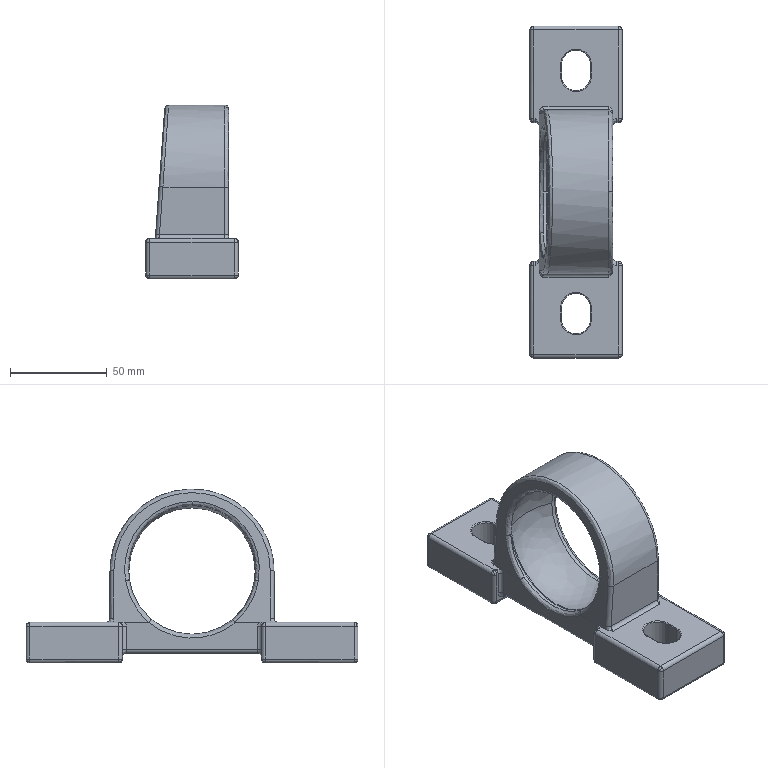Part | SolidWorks | features BaseBody 1 | 1 solid | 147 faces | box 48 x 172 x 90.1 mm | volume 179022 mm3 | spline 68 | cylinder 57 | plane 22 | commonest cylinder face diameters 4 x40 1 x8 15 x4 65.452 x4 85 x1